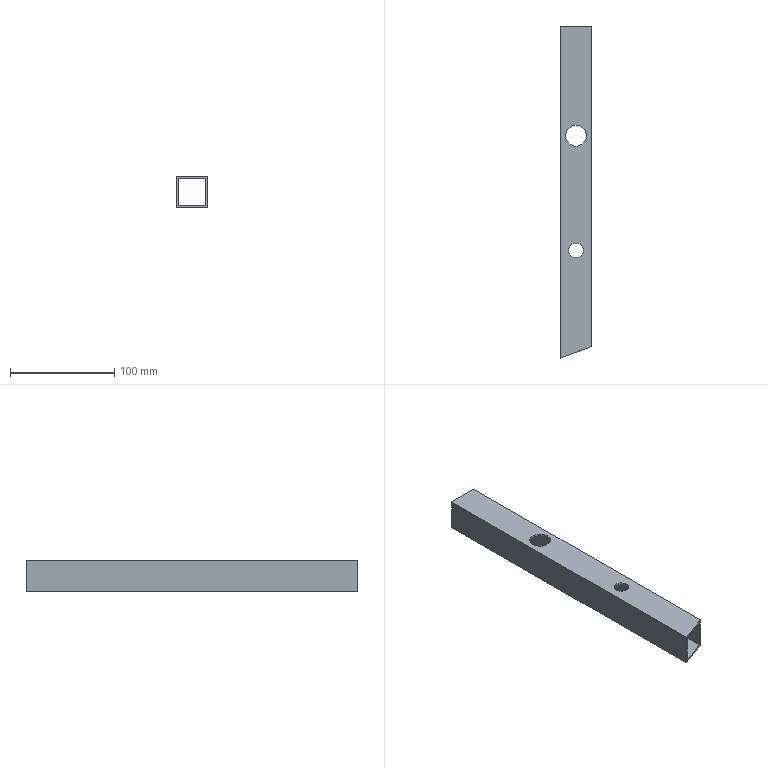Part | NX | features solid 2 | 1 solid | 14 faces | box 30 x 317.844 x 30 mm | volume 68102 mm3 | plane 10 | cylinder 4 | commonest cylinder face diameters 14 x2 20 x2
STEP:
#1=CARTESIAN_POINT('',(680.,25.,0.));
#2=VERTEX_POINT('',#1);
#3=CARTESIAN_POINT('',(680.,-281.925,0.));
#4=VERTEX_POINT('',#3);
#5=CARTESIAN_POINT('',(680.,-30.,0.));
#6=DIRECTION('',(0.,-1.,0.));
#7=VECTOR('',#6,1000.);
#8=LINE('',#5,#7);
#9=EDGE_CURVE('',#2,#4,#8,.T.);
#10=ORIENTED_EDGE('',*,*,#9,.F.);
#11=CARTESIAN_POINT('',(650.,25.,0.));
#12=VERTEX_POINT('',#11);
#13=CARTESIAN_POINT('',(681.,25.,0.));
#14=DIRECTION('',(-1.,0.,0.));
#15=VECTOR('',#14,1000.);
#16=LINE('',#13,#15);
#17=EDGE_CURVE('',#2,#12,#16,.T.);
#18=ORIENTED_EDGE('',*,*,#17,.T.);
#19=CARTESIAN_POINT('',(650.,-292.844,0.));
#20=VERTEX_POINT('',#19);
#21=CARTESIAN_POINT('',(650.,-30.,0.));
#22=DIRECTION('',(0.,1.,0.));
#23=VECTOR('',#22,1000.);
#24=LINE('',#21,#23);
#25=EDGE_CURVE('',#12,#20,#24,.F.);
#26=ORIENTED_EDGE('',*,*,#25,.T.);
#27=CARTESIAN_POINT('',(761.85,-252.134,0.));
#28=DIRECTION('',(0.9397,0.342,0.));
#29=VECTOR('',#28,1000.);
#30=LINE('',#27,#29);
#31=EDGE_CURVE('',#4,#20,#30,.F.);
#32=ORIENTED_EDGE('',*,*,#31,.F.);
#33=EDGE_LOOP('',(#10,#18,#26,#32));
#34=FACE_BOUND('',#33,.T.);
#35=CARTESIAN_POINT('',(675.,-80.,0.));
#36=VERTEX_POINT('',#35);
#37=CARTESIAN_POINT('',(665.,-80.,0.));
#38=DIRECTION('',(0.,0.,1.));
#39=DIRECTION('',(1.,0.,0.));
#40=AXIS2_PLACEMENT_3D('',#37,#38,#39);
#41=CIRCLE('',#40,10.);
#42=EDGE_CURVE('',#36,#36,#41,.F.);
#43=ORIENTED_EDGE('',*,*,#42,.T.);
#44=EDGE_LOOP('',(#43));
#45=FACE_BOUND('',#44,.T.);
#46=CARTESIAN_POINT('',(672.,-190.,0.));
#47=VERTEX_POINT('',#46);
#48=CARTESIAN_POINT('',(665.,-190.,0.));
#49=DIRECTION('',(0.,0.,1.));
#50=DIRECTION('',(1.,0.,0.));
#51=AXIS2_PLACEMENT_3D('',#48,#49,#50);
#52=CIRCLE('',#51,7.);
#53=EDGE_CURVE('',#47,#47,#52,.F.);
#54=ORIENTED_EDGE('',*,*,#53,.T.);
#55=EDGE_LOOP('',(#54));
#56=FACE_BOUND('',#55,.T.);
#57=CARTESIAN_POINT('',(681.,-30.,0.));
#58=DIRECTION('',(0.,0.,1.));
#59=DIRECTION('',(-1.,0.,0.));
#60=AXIS2_PLACEMENT_3D('',#57,#58,#59);
#61=PLANE('',#60);
#62=ADVANCED_FACE('',(#34,#45,#56),#61,.T.);
#63=CARTESIAN_POINT('',(680.,25.,-30.));
#64=VERTEX_POINT('',#63);
#65=CARTESIAN_POINT('',(650.,25.,-30.));
#66=VERTEX_POINT('',#65);
#67=CARTESIAN_POINT('',(681.,25.,-30.));
#68=DIRECTION('',(-1.,0.,0.));
#69=VECTOR('',#68,1000.);
#70=LINE('',#67,#69);
#71=EDGE_CURVE('',#64,#66,#70,.T.);
#72=ORIENTED_EDGE('',*,*,#71,.F.);
#73=CARTESIAN_POINT('',(680.,-281.925,-30.));
#74=VERTEX_POINT('',#73);
#75=CARTESIAN_POINT('',(680.,-30.,-30.));
#76=DIRECTION('',(0.,-1.,0.));
#77=VECTOR('',#76,1000.);
#78=LINE('',#75,#77);
#79=EDGE_CURVE('',#64,#74,#78,.T.);
#80=ORIENTED_EDGE('',*,*,#79,.T.);
#81=CARTESIAN_POINT('',(650.,-292.844,-30.));
#82=VERTEX_POINT('',#81);
#83=CARTESIAN_POINT('',(761.85,-252.134,-30.));
#84=DIRECTION('',(0.9397,0.342,0.));
#85=VECTOR('',#84,1000.);
#86=LINE('',#83,#85);
#87=EDGE_CURVE('',#74,#82,#86,.F.);
#88=ORIENTED_EDGE('',*,*,#87,.T.);
#89=CARTESIAN_POINT('',(650.,-30.,-30.));
#90=DIRECTION('',(0.,1.,0.));
#91=VECTOR('',#90,1000.);
#92=LINE('',#89,#91);
#93=EDGE_CURVE('',#66,#82,#92,.F.);
#94=ORIENTED_EDGE('',*,*,#93,.F.);
#95=EDGE_LOOP('',(#72,#80,#88,#94));
#96=FACE_BOUND('',#95,.T.);
#97=CARTESIAN_POINT('',(675.,-80.,-30.));
#98=VERTEX_POINT('',#97);
#99=CARTESIAN_POINT('',(665.,-80.,-30.));
#100=DIRECTION('',(0.,0.,1.));
#101=DIRECTION('',(1.,0.,0.));
#102=AXIS2_PLACEMENT_3D('',#99,#100,#101);
#103=CIRCLE('',#102,10.);
#104=EDGE_CURVE('',#98,#98,#103,.T.);
#105=ORIENTED_EDGE('',*,*,#104,.T.);
#106=EDGE_LOOP('',(#105));
#107=FACE_BOUND('',#106,.T.);
#108=CARTESIAN_POINT('',(672.,-190.,-30.));
#109=VERTEX_POINT('',#108);
#110=CARTESIAN_POINT('',(665.,-190.,-30.));
#111=DIRECTION('',(0.,0.,1.));
#112=DIRECTION('',(1.,0.,0.));
#113=AXIS2_PLACEMENT_3D('',#110,#111,#112);
#114=CIRCLE('',#113,7.);
#115=EDGE_CURVE('',#109,#109,#114,.T.);
#116=ORIENTED_EDGE('',*,*,#115,.T.);
#117=EDGE_LOOP('',(#116));
#118=FACE_BOUND('',#117,.T.);
#119=CARTESIAN_POINT('',(681.,-30.,-30.));
#120=DIRECTION('',(0.,0.,1.));
#121=DIRECTION('',(-1.,0.,0.));
#122=AXIS2_PLACEMENT_3D('',#119,#120,#121);
#123=PLANE('',#122);
#124=ADVANCED_FACE('',(#96,#107,#118),#123,.F.);
#125=CARTESIAN_POINT('',(652.,25.,-28.));
#126=VERTEX_POINT('',#125);
#127=CARTESIAN_POINT('',(678.,25.,-28.));
#128=VERTEX_POINT('',#127);
#129=CARTESIAN_POINT('',(681.,25.,-28.));
#130=DIRECTION('',(1.,0.,0.));
#131=VECTOR('',#130,1000.);
#132=LINE('',#129,#131);
#133=EDGE_CURVE('',#126,#128,#132,.T.);
#134=ORIENTED_EDGE('',*,*,#133,.F.);
#135=CARTESIAN_POINT('',(652.,-292.116,-28.));
#136=VERTEX_POINT('',#135);
#137=CARTESIAN_POINT('',(652.,-455.,-28.));
#138=DIRECTION('',(0.,1.,0.));
#139=VECTOR('',#138,1000.);
#140=LINE('',#137,#139);
#141=EDGE_CURVE('',#136,#126,#140,.T.);
#142=ORIENTED_EDGE('',*,*,#141,.F.);
#143=CARTESIAN_POINT('',(678.,-282.653,-28.));
#144=VERTEX_POINT('',#143);
#145=CARTESIAN_POINT('',(690.261,-278.191,-28.));
#146=DIRECTION('',(0.9397,0.342,0.));
#147=VECTOR('',#146,1000.);
#148=LINE('',#145,#147);
#149=EDGE_CURVE('',#144,#136,#148,.F.);
#150=ORIENTED_EDGE('',*,*,#149,.F.);
#151=CARTESIAN_POINT('',(678.,-455.,-28.));
#152=DIRECTION('',(0.,1.,0.));
#153=VECTOR('',#152,1000.);
#154=LINE('',#151,#153);
#155=EDGE_CURVE('',#144,#128,#154,.T.);
#156=ORIENTED_EDGE('',*,*,#155,.T.);
#157=EDGE_LOOP('',(#134,#142,#150,#156));
#158=FACE_BOUND('',#157,.T.);
#159=CARTESIAN_POINT('',(655.,-80.,-28.));
#160=VERTEX_POINT('',#159);
#161=CARTESIAN_POINT('',(665.,-80.,-28.));
#162=DIRECTION('',(0.,0.,-1.));
#163=DIRECTION('',(-1.,0.,0.));
#164=AXIS2_PLACEMENT_3D('',#161,#162,#163);
#165=CIRCLE('',#164,10.);
#166=EDGE_CURVE('',#160,#160,#165,.T.);
#167=ORIENTED_EDGE('',*,*,#166,.T.);
#168=EDGE_LOOP('',(#167));
#169=FACE_BOUND('',#168,.T.);
#170=CARTESIAN_POINT('',(658.,-190.,-28.));
#171=VERTEX_POINT('',#170);
#172=CARTESIAN_POINT('',(665.,-190.,-28.));
#173=DIRECTION('',(0.,0.,-1.));
#174=DIRECTION('',(-1.,0.,0.));
#175=AXIS2_PLACEMENT_3D('',#172,#173,#174);
#176=CIRCLE('',#175,7.);
#177=EDGE_CURVE('',#171,#171,#176,.F.);
#178=ORIENTED_EDGE('',*,*,#177,.F.);
#179=EDGE_LOOP('',(#178));
#180=FACE_BOUND('',#179,.T.);
#181=CARTESIAN_POINT('',(681.,-455.,-28.));
#182=DIRECTION('',(0.,0.,-1.));
#183=DIRECTION('',(1.,0.,0.));
#184=AXIS2_PLACEMENT_3D('',#181,#182,#183);
#185=PLANE('',#184);
#186=ADVANCED_FACE('',(#158,#169,#180),#185,.F.);
#187=CARTESIAN_POINT('',(652.,-292.116,-2.));
#188=VERTEX_POINT('',#187);
#189=CARTESIAN_POINT('',(652.,25.,-2.));
#190=VERTEX_POINT('',#189);
#191=CARTESIAN_POINT('',(652.,-455.,-2.));
#192=DIRECTION('',(0.,1.,0.));
#193=VECTOR('',#192,1000.);
#194=LINE('',#191,#193);
#195=EDGE_CURVE('',#188,#190,#194,.T.);
#196=ORIENTED_EDGE('',*,*,#195,.T.);
#197=CARTESIAN_POINT('',(678.,25.,-2.));
#198=VERTEX_POINT('',#197);
#199=CARTESIAN_POINT('',(681.,25.,-2.));
#200=DIRECTION('',(1.,0.,0.));
#201=VECTOR('',#200,1000.);
#202=LINE('',#199,#201);
#203=EDGE_CURVE('',#190,#198,#202,.T.);
#204=ORIENTED_EDGE('',*,*,#203,.T.);
#205=CARTESIAN_POINT('',(678.,-282.653,-2.));
#206=VERTEX_POINT('',#205);
#207=CARTESIAN_POINT('',(678.,-455.,-2.));
#208=DIRECTION('',(0.,1.,0.));
#209=VECTOR('',#208,1000.);
#210=LINE('',#207,#209);
#211=EDGE_CURVE('',#206,#198,#210,.T.);
#212=ORIENTED_EDGE('',*,*,#211,.F.);
#213=CARTESIAN_POINT('',(690.261,-278.191,-2.));
#214=DIRECTION('',(0.9397,0.342,0.));
#215=VECTOR('',#214,1000.);
#216=LINE('',#213,#215);
#217=EDGE_CURVE('',#206,#188,#216,.F.);
#218=ORIENTED_EDGE('',*,*,#217,.T.);
#219=EDGE_LOOP('',(#196,#204,#212,#218));
#220=FACE_BOUND('',#219,.T.);
#221=CARTESIAN_POINT('',(655.,-80.,-2.));
#222=VERTEX_POINT('',#221);
#223=CARTESIAN_POINT('',(665.,-80.,-2.));
#224=DIRECTION('',(0.,0.,-1.));
#225=DIRECTION('',(-1.,0.,0.));
#226=AXIS2_PLACEMENT_3D('',#223,#224,#225);
#227=CIRCLE('',#226,10.);
#228=EDGE_CURVE('',#222,#222,#227,.T.);
#229=ORIENTED_EDGE('',*,*,#228,.F.);
#230=EDGE_LOOP('',(#229));
#231=FACE_BOUND('',#230,.T.);
#232=CARTESIAN_POINT('',(658.,-190.,-2.));
#233=VERTEX_POINT('',#232);
#234=CARTESIAN_POINT('',(665.,-190.,-2.));
#235=DIRECTION('',(0.,0.,-1.));
#236=DIRECTION('',(-1.,0.,0.));
#237=AXIS2_PLACEMENT_3D('',#234,#235,#236);
#238=CIRCLE('',#237,7.);
#239=EDGE_CURVE('',#233,#233,#238,.F.);
#240=ORIENTED_EDGE('',*,*,#239,.T.);
#241=EDGE_LOOP('',(#240));
#242=FACE_BOUND('',#241,.T.);
#243=CARTESIAN_POINT('',(681.,-455.,-2.));
#244=DIRECTION('',(0.,0.,-1.));
#245=DIRECTION('',(1.,0.,0.));
#246=AXIS2_PLACEMENT_3D('',#243,#244,#245);
#247=PLANE('',#246);
#248=ADVANCED_FACE('',(#220,#231,#242),#247,.T.);
#249=CARTESIAN_POINT('',(650.,25.,-25.));
#250=DIRECTION('',(0.,0.,-1.));
#251=VECTOR('',#250,1000.);
#252=LINE('',#249,#251);
#253=EDGE_CURVE('',#66,#12,#252,.F.);
#254=ORIENTED_EDGE('',*,*,#253,.F.);
#255=ORIENTED_EDGE('',*,*,#93,.T.);
#256=CARTESIAN_POINT('',(650.,-292.844,0.));
#257=DIRECTION('',(0.,0.,-1.));
#258=VECTOR('',#257,1000.);
#259=LINE('',#256,#258);
#260=EDGE_CURVE('',#20,#82,#259,.T.);
#261=ORIENTED_EDGE('',*,*,#260,.F.);
#262=ORIENTED_EDGE('',*,*,#25,.F.);
#263=EDGE_LOOP('',(#254,#255,#261,#262));
#264=FACE_BOUND('',#263,.T.);
#265=CARTESIAN_POINT('',(650.,-30.,-25.));
#266=DIRECTION('',(-1.,0.,0.));
#267=DIRECTION('',(0.,-1.,0.));
#268=AXIS2_PLACEMENT_3D('',#265,#266,#267);
#269=PLANE('',#268);
#270=ADVANCED_FACE('',(#264),#269,.T.);
#271=CARTESIAN_POINT('',(680.,25.,-25.));
#272=DIRECTION('',(0.,0.,-1.));
#273=VECTOR('',#272,1000.);
#274=LINE('',#271,#273);
#275=EDGE_CURVE('',#2,#64,#274,.T.);
#276=ORIENTED_EDGE('',*,*,#275,.F.);
#277=ORIENTED_EDGE('',*,*,#9,.T.);
#278=CARTESIAN_POINT('',(680.,-281.925,-25.));
#279=DIRECTION('',(0.,0.,1.));
#280=VECTOR('',#279,1000.);
#281=LINE('',#278,#280);
#282=EDGE_CURVE('',#4,#74,#281,.F.);
#283=ORIENTED_EDGE('',*,*,#282,.T.);
#284=ORIENTED_EDGE('',*,*,#79,.F.);
#285=EDGE_LOOP('',(#276,#277,#283,#284));
#286=FACE_BOUND('',#285,.T.);
#287=CARTESIAN_POINT('',(680.,-30.,-25.));
#288=DIRECTION('',(-1.,0.,0.));
#289=DIRECTION('',(0.,-1.,0.));
#290=AXIS2_PLACEMENT_3D('',#287,#288,#289);
#291=PLANE('',#290);
#292=ADVANCED_FACE('',(#286),#291,.F.);
#293=CARTESIAN_POINT('',(678.,25.,-25.));
#294=DIRECTION('',(0.,0.,1.));
#295=VECTOR('',#294,1000.);
#296=LINE('',#293,#295);
#297=EDGE_CURVE('',#128,#198,#296,.T.);
#298=ORIENTED_EDGE('',*,*,#297,.F.);
#299=ORIENTED_EDGE('',*,*,#155,.F.);
#300=CARTESIAN_POINT('',(678.,-282.653,0.));
#301=DIRECTION('',(0.,0.,1.));
#302=VECTOR('',#301,1000.);
#303=LINE('',#300,#302);
#304=EDGE_CURVE('',#206,#144,#303,.F.);
#305=ORIENTED_EDGE('',*,*,#304,.F.);
#306=ORIENTED_EDGE('',*,*,#211,.T.);
#307=EDGE_LOOP('',(#298,#299,#305,#306));
#308=FACE_BOUND('',#307,.T.);
#309=CARTESIAN_POINT('',(678.,-455.,-25.));
#310=DIRECTION('',(1.,0.,0.));
#311=DIRECTION('',(0.,0.,1.));
#312=AXIS2_PLACEMENT_3D('',#309,#310,#311);
#313=PLANE('',#312);
#314=ADVANCED_FACE('',(#308),#313,.F.);
#315=ORIENTED_EDGE('',*,*,#141,.T.);
#316=CARTESIAN_POINT('',(652.,25.,-25.));
#317=DIRECTION('',(0.,0.,1.));
#318=VECTOR('',#317,1000.);
#319=LINE('',#316,#318);
#320=EDGE_CURVE('',#126,#190,#319,.T.);
#321=ORIENTED_EDGE('',*,*,#320,.T.);
#322=ORIENTED_EDGE('',*,*,#195,.F.);
#323=CARTESIAN_POINT('',(652.,-292.116,0.));
#324=DIRECTION('',(0.,0.,1.));
#325=VECTOR('',#324,1000.);
#326=LINE('',#323,#325);
#327=EDGE_CURVE('',#188,#136,#326,.F.);
#328=ORIENTED_EDGE('',*,*,#327,.T.);
#329=EDGE_LOOP('',(#315,#321,#322,#328));
#330=FACE_BOUND('',#329,.T.);
#331=CARTESIAN_POINT('',(652.,-455.,-25.));
#332=DIRECTION('',(1.,0.,0.));
#333=DIRECTION('',(0.,0.,1.));
#334=AXIS2_PLACEMENT_3D('',#331,#332,#333);
#335=PLANE('',#334);
#336=ADVANCED_FACE('',(#330),#335,.T.);
#337=ORIENTED_EDGE('',*,*,#42,.F.);
#338=EDGE_LOOP('',(#337));
#339=FACE_BOUND('',#338,.T.);
#340=ORIENTED_EDGE('',*,*,#228,.T.);
#341=EDGE_LOOP('',(#340));
#342=FACE_BOUND('',#341,.T.);
#343=CARTESIAN_POINT('',(665.,-80.,28.));
#344=DIRECTION('',(0.,0.,-1.));
#345=DIRECTION('',(1.,0.,0.));
#346=AXIS2_PLACEMENT_3D('',#343,#344,#345);
#347=CYLINDRICAL_SURFACE('',#346,10.);
#348=ADVANCED_FACE('',(#339,#342),#347,.F.);
#349=ORIENTED_EDGE('',*,*,#217,.F.);
#350=ORIENTED_EDGE('',*,*,#304,.T.);
#351=ORIENTED_EDGE('',*,*,#149,.T.);
#352=ORIENTED_EDGE('',*,*,#327,.F.);
#353=EDGE_LOOP('',(#349,#350,#351,#352));
#354=FACE_BOUND('',#353,.T.);
#355=ORIENTED_EDGE('',*,*,#260,.T.);
#356=ORIENTED_EDGE('',*,*,#87,.F.);
#357=ORIENTED_EDGE('',*,*,#282,.F.);
#358=ORIENTED_EDGE('',*,*,#31,.T.);
#359=EDGE_LOOP('',(#355,#356,#357,#358));
#360=FACE_BOUND('',#359,.T.);
#361=CARTESIAN_POINT('',(690.261,-278.191,0.));
#362=DIRECTION('',(0.342,-0.9397,0.));
#363=DIRECTION('',(-0.9397,-0.342,0.));
#364=AXIS2_PLACEMENT_3D('',#361,#362,#363);
#365=PLANE('',#364);
#366=ADVANCED_FACE('',(#354,#360),#365,.T.);
#367=ORIENTED_EDGE('',*,*,#166,.F.);
#368=EDGE_LOOP('',(#367));
#369=FACE_BOUND('',#368,.T.);
#370=ORIENTED_EDGE('',*,*,#104,.F.);
#371=EDGE_LOOP('',(#370));
#372=FACE_BOUND('',#371,.T.);
#373=CARTESIAN_POINT('',(665.,-80.,28.));
#374=DIRECTION('',(0.,0.,-1.));
#375=DIRECTION('',(1.,0.,0.));
#376=AXIS2_PLACEMENT_3D('',#373,#374,#375);
#377=CYLINDRICAL_SURFACE('',#376,10.);
#378=ADVANCED_FACE('',(#369,#372),#377,.F.);
#379=ORIENTED_EDGE('',*,*,#320,.F.);
#380=ORIENTED_EDGE('',*,*,#133,.T.);
#381=ORIENTED_EDGE('',*,*,#297,.T.);
#382=ORIENTED_EDGE('',*,*,#203,.F.);
#383=EDGE_LOOP('',(#379,#380,#381,#382));
#384=FACE_BOUND('',#383,.T.);
#385=ORIENTED_EDGE('',*,*,#71,.T.);
#386=ORIENTED_EDGE('',*,*,#253,.T.);
#387=ORIENTED_EDGE('',*,*,#17,.F.);
#388=ORIENTED_EDGE('',*,*,#275,.T.);
#389=EDGE_LOOP('',(#385,#386,#387,#388));
#390=FACE_BOUND('',#389,.T.);
#391=CARTESIAN_POINT('',(660.,25.,0.));
#392=DIRECTION('',(0.,1.,0.));
#393=DIRECTION('',(0.,0.,1.));
#394=AXIS2_PLACEMENT_3D('',#391,#392,#393);
#395=PLANE('',#394);
#396=ADVANCED_FACE('',(#384,#390),#395,.T.);
#397=ORIENTED_EDGE('',*,*,#53,.F.);
#398=EDGE_LOOP('',(#397));
#399=FACE_BOUND('',#398,.T.);
#400=ORIENTED_EDGE('',*,*,#239,.F.);
#401=EDGE_LOOP('',(#400));
#402=FACE_BOUND('',#401,.T.);
#403=CARTESIAN_POINT('',(665.,-190.,-25.));
#404=DIRECTION('',(0.,0.,-1.));
#405=DIRECTION('',(1.,0.,0.));
#406=AXIS2_PLACEMENT_3D('',#403,#404,#405);
#407=CYLINDRICAL_SURFACE('',#406,7.);
#408=ADVANCED_FACE('',(#399,#402),#407,.F.);
#409=ORIENTED_EDGE('',*,*,#115,.F.);
#410=EDGE_LOOP('',(#409));
#411=FACE_BOUND('',#410,.T.);
#412=ORIENTED_EDGE('',*,*,#177,.T.);
#413=EDGE_LOOP('',(#412));
#414=FACE_BOUND('',#413,.T.);
#415=CARTESIAN_POINT('',(665.,-190.,-25.));
#416=DIRECTION('',(0.,0.,-1.));
#417=DIRECTION('',(1.,0.,0.));
#418=AXIS2_PLACEMENT_3D('',#415,#416,#417);
#419=CYLINDRICAL_SURFACE('',#418,7.);
#420=ADVANCED_FACE('',(#411,#414),#419,.F.);
#421=CLOSED_SHELL('',(#62,#124,#186,#248,#270,#292,#314,#336,#348,#366,#378,#396,#408,#420));
#422=MANIFOLD_SOLID_BREP('',#421);
#423=(LENGTH_UNIT()NAMED_UNIT(*)SI_UNIT(.MILLI.,.METRE.));
#424=UNCERTAINTY_MEASURE_WITH_UNIT(LENGTH_MEASURE(0.00001),#423,'','');
#425=(NAMED_UNIT(*)PLANE_ANGLE_UNIT()SI_UNIT($,.RADIAN.));
#426=(NAMED_UNIT(*)SI_UNIT($,.STERADIAN.)SOLID_ANGLE_UNIT());
#427=(GEOMETRIC_REPRESENTATION_CONTEXT(3)GLOBAL_UNCERTAINTY_ASSIGNED_CONTEXT((#424))GLOBAL_UNIT_ASSIGNED_CONTEXT((#423,#425,#426))REPRESENTATION_CONTEXT('',''));
#428=ADVANCED_BREP_SHAPE_REPRESENTATION('',(#422),#427);